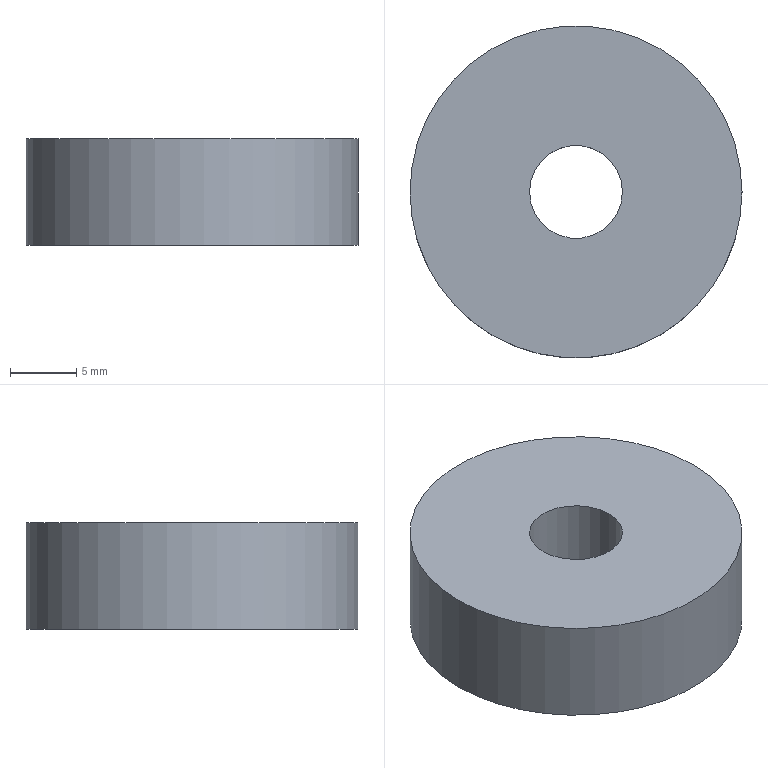Part | NX | 1 solid | 9 faces | box 25 x 25 x 8 mm | volume 3366 mm3 | cylinder 4 | plane 4 | cone 1 | commonest cylinder face diameters 7 x1 21.2 x1 21.8 x1 25 x1
STEP:
#1=CARTESIAN_POINT('',(12.5,0.,-8.));
#2=VERTEX_POINT('',#1);
#3=CARTESIAN_POINT('',(0.,0.,-8.));
#4=DIRECTION('',(0.,0.,1.));
#5=DIRECTION('',(1.,0.,0.));
#6=AXIS2_PLACEMENT_3D('',#3,#4,#5);
#7=CIRCLE('',#6,12.5);
#8=EDGE_CURVE('',#2,#2,#7,.T.);
#9=ORIENTED_EDGE('',*,*,#8,.T.);
#10=EDGE_LOOP('',(#9));
#11=FACE_BOUND('',#10,.T.);
#12=CARTESIAN_POINT('',(12.5,0.,0.));
#13=VERTEX_POINT('',#12);
#14=CARTESIAN_POINT('',(0.,0.,0.));
#15=DIRECTION('',(0.,0.,1.));
#16=DIRECTION('',(1.,0.,0.));
#17=AXIS2_PLACEMENT_3D('',#14,#15,#16);
#18=CIRCLE('',#17,12.5);
#19=EDGE_CURVE('',#13,#13,#18,.F.);
#20=ORIENTED_EDGE('',*,*,#19,.T.);
#21=EDGE_LOOP('',(#20));
#22=FACE_BOUND('',#21,.T.);
#23=CARTESIAN_POINT('',(0.,0.,-8.));
#24=DIRECTION('',(0.,0.,1.));
#25=DIRECTION('',(1.,0.,0.));
#26=AXIS2_PLACEMENT_3D('',#23,#24,#25);
#27=CYLINDRICAL_SURFACE('',#26,12.5);
#28=ADVANCED_FACE('',(#11,#22),#27,.T.);
#29=CARTESIAN_POINT('',(10.9,0.,-8.));
#30=VERTEX_POINT('',#29);
#31=CARTESIAN_POINT('',(0.,0.,-8.));
#32=DIRECTION('',(0.,0.,1.));
#33=DIRECTION('',(1.,0.,0.));
#34=AXIS2_PLACEMENT_3D('',#31,#32,#33);
#35=CIRCLE('',#34,10.9);
#36=EDGE_CURVE('',#30,#30,#35,.T.);
#37=ORIENTED_EDGE('',*,*,#36,.T.);
#38=EDGE_LOOP('',(#37));
#39=FACE_BOUND('',#38,.T.);
#40=ORIENTED_EDGE('',*,*,#8,.F.);
#41=EDGE_LOOP('',(#40));
#42=FACE_BOUND('',#41,.T.);
#43=CARTESIAN_POINT('',(0.,10.9,-8.));
#44=DIRECTION('',(0.,0.,-1.));
#45=DIRECTION('',(-1.,0.,0.));
#46=AXIS2_PLACEMENT_3D('',#43,#44,#45);
#47=PLANE('',#46);
#48=ADVANCED_FACE('',(#39,#42),#47,.T.);
#49=ORIENTED_EDGE('',*,*,#19,.F.);
#50=EDGE_LOOP('',(#49));
#51=FACE_BOUND('',#50,.T.);
#52=CARTESIAN_POINT('',(3.5,0.,0.));
#53=VERTEX_POINT('',#52);
#54=CARTESIAN_POINT('',(0.,0.,0.));
#55=DIRECTION('',(0.,0.,1.));
#56=DIRECTION('',(1.,0.,0.));
#57=AXIS2_PLACEMENT_3D('',#54,#55,#56);
#58=CIRCLE('',#57,3.5);
#59=EDGE_CURVE('',#53,#53,#58,.F.);
#60=ORIENTED_EDGE('',*,*,#59,.T.);
#61=EDGE_LOOP('',(#60));
#62=FACE_BOUND('',#61,.T.);
#63=CARTESIAN_POINT('',(0.,12.5,0.));
#64=DIRECTION('',(0.,0.,1.));
#65=DIRECTION('',(1.,0.,0.));
#66=AXIS2_PLACEMENT_3D('',#63,#64,#65);
#67=PLANE('',#66);
#68=ADVANCED_FACE('',(#51,#62),#67,.T.);
#69=CARTESIAN_POINT('',(10.9,0.,-1.8));
#70=VERTEX_POINT('',#69);
#71=CARTESIAN_POINT('',(0.,0.,-1.8));
#72=DIRECTION('',(0.,0.,1.));
#73=DIRECTION('',(1.,0.,0.));
#74=AXIS2_PLACEMENT_3D('',#71,#72,#73);
#75=CIRCLE('',#74,10.9);
#76=EDGE_CURVE('',#70,#70,#75,.F.);
#77=ORIENTED_EDGE('',*,*,#76,.F.);
#78=EDGE_LOOP('',(#77));
#79=FACE_BOUND('',#78,.T.);
#80=ORIENTED_EDGE('',*,*,#36,.F.);
#81=EDGE_LOOP('',(#80));
#82=FACE_BOUND('',#81,.T.);
#83=CARTESIAN_POINT('',(0.,0.,-8.));
#84=DIRECTION('',(0.,0.,1.));
#85=DIRECTION('',(1.,0.,0.));
#86=AXIS2_PLACEMENT_3D('',#83,#84,#85);
#87=CYLINDRICAL_SURFACE('',#86,10.9);
#88=ADVANCED_FACE('',(#79,#82),#87,.F.);
#89=ORIENTED_EDGE('',*,*,#59,.F.);
#90=EDGE_LOOP('',(#89));
#91=FACE_BOUND('',#90,.T.);
#92=CARTESIAN_POINT('',(-3.5,0.,-5.));
#93=VERTEX_POINT('',#92);
#94=CARTESIAN_POINT('',(0.,0.,-5.));
#95=DIRECTION('',(0.,0.,1.));
#96=DIRECTION('',(1.,0.,0.));
#97=AXIS2_PLACEMENT_3D('',#94,#95,#96);
#98=CIRCLE('',#97,3.5);
#99=EDGE_CURVE('',#93,#93,#98,.T.);
#100=ORIENTED_EDGE('',*,*,#99,.F.);
#101=EDGE_LOOP('',(#100));
#102=FACE_BOUND('',#101,.T.);
#103=CARTESIAN_POINT('',(0.,0.,-8.));
#104=DIRECTION('',(0.,0.,1.));
#105=DIRECTION('',(1.,0.,0.));
#106=AXIS2_PLACEMENT_3D('',#103,#104,#105);
#107=CYLINDRICAL_SURFACE('',#106,3.5);
#108=ADVANCED_FACE('',(#91,#102),#107,.F.);
#109=CARTESIAN_POINT('',(10.6,0.,-1.8));
#110=VERTEX_POINT('',#109);
#111=CARTESIAN_POINT('',(0.,0.,-1.8));
#112=DIRECTION('',(0.,0.,1.));
#113=DIRECTION('',(1.,0.,0.));
#114=AXIS2_PLACEMENT_3D('',#111,#112,#113);
#115=CIRCLE('',#114,10.6);
#116=EDGE_CURVE('',#110,#110,#115,.T.);
#117=ORIENTED_EDGE('',*,*,#116,.T.);
#118=EDGE_LOOP('',(#117));
#119=FACE_BOUND('',#118,.T.);
#120=ORIENTED_EDGE('',*,*,#76,.T.);
#121=EDGE_LOOP('',(#120));
#122=FACE_BOUND('',#121,.T.);
#123=CARTESIAN_POINT('',(0.,10.6,-1.8));
#124=DIRECTION('',(0.,0.,-1.));
#125=DIRECTION('',(-1.,0.,0.));
#126=AXIS2_PLACEMENT_3D('',#123,#124,#125);
#127=PLANE('',#126);
#128=ADVANCED_FACE('',(#119,#122),#127,.T.);
#129=ORIENTED_EDGE('',*,*,#99,.T.);
#130=EDGE_LOOP('',(#129));
#131=FACE_BOUND('',#130,.T.);
#132=CARTESIAN_POINT('',(-6.5,0.,-8.));
#133=VERTEX_POINT('',#132);
#134=CARTESIAN_POINT('',(0.,0.,-8.));
#135=DIRECTION('',(0.,0.,-1.));
#136=DIRECTION('',(-1.,0.,0.));
#137=AXIS2_PLACEMENT_3D('',#134,#135,#136);
#138=CIRCLE('',#137,6.5);
#139=EDGE_CURVE('',#133,#133,#138,.F.);
#140=ORIENTED_EDGE('',*,*,#139,.F.);
#141=EDGE_LOOP('',(#140));
#142=FACE_BOUND('',#141,.T.);
#143=CARTESIAN_POINT('',(0.,0.,-8.));
#144=DIRECTION('',(0.,0.,-1.));
#145=DIRECTION('',(-1.,0.,0.));
#146=AXIS2_PLACEMENT_3D('',#143,#144,#145);
#147=CONICAL_SURFACE('',#146,6.5,0.7854);
#148=ADVANCED_FACE('',(#131,#142),#147,.F.);
#149=CARTESIAN_POINT('',(10.6,0.,-8.));
#150=VERTEX_POINT('',#149);
#151=CARTESIAN_POINT('',(0.,0.,-8.));
#152=DIRECTION('',(0.,0.,1.));
#153=DIRECTION('',(1.,0.,0.));
#154=AXIS2_PLACEMENT_3D('',#151,#152,#153);
#155=CIRCLE('',#154,10.6);
#156=EDGE_CURVE('',#150,#150,#155,.T.);
#157=ORIENTED_EDGE('',*,*,#156,.T.);
#158=EDGE_LOOP('',(#157));
#159=FACE_BOUND('',#158,.T.);
#160=ORIENTED_EDGE('',*,*,#116,.F.);
#161=EDGE_LOOP('',(#160));
#162=FACE_BOUND('',#161,.T.);
#163=CARTESIAN_POINT('',(0.,0.,-8.));
#164=DIRECTION('',(0.,0.,1.));
#165=DIRECTION('',(1.,0.,0.));
#166=AXIS2_PLACEMENT_3D('',#163,#164,#165);
#167=CYLINDRICAL_SURFACE('',#166,10.6);
#168=ADVANCED_FACE('',(#159,#162),#167,.T.);
#169=ORIENTED_EDGE('',*,*,#139,.T.);
#170=EDGE_LOOP('',(#169));
#171=FACE_BOUND('',#170,.T.);
#172=ORIENTED_EDGE('',*,*,#156,.F.);
#173=EDGE_LOOP('',(#172));
#174=FACE_BOUND('',#173,.T.);
#175=CARTESIAN_POINT('',(0.,6.5,-8.));
#176=DIRECTION('',(0.,0.,-1.));
#177=DIRECTION('',(-1.,0.,0.));
#178=AXIS2_PLACEMENT_3D('',#175,#176,#177);
#179=PLANE('',#178);
#180=ADVANCED_FACE('',(#171,#174),#179,.T.);
#181=CLOSED_SHELL('',(#28,#48,#68,#88,#108,#128,#148,#168,#180));
#182=MANIFOLD_SOLID_BREP('',#181);
#183=(LENGTH_UNIT()NAMED_UNIT(*)SI_UNIT(.MILLI.,.METRE.));
#184=UNCERTAINTY_MEASURE_WITH_UNIT(LENGTH_MEASURE(0.00001),#183,'','');
#185=(NAMED_UNIT(*)PLANE_ANGLE_UNIT()SI_UNIT($,.RADIAN.));
#186=(NAMED_UNIT(*)SI_UNIT($,.STERADIAN.)SOLID_ANGLE_UNIT());
#187=(GEOMETRIC_REPRESENTATION_CONTEXT(3)GLOBAL_UNCERTAINTY_ASSIGNED_CONTEXT((#184))GLOBAL_UNIT_ASSIGNED_CONTEXT((#183,#185,#186))REPRESENTATION_CONTEXT('',''));
#188=ADVANCED_BREP_SHAPE_REPRESENTATION('',(#182),#187);